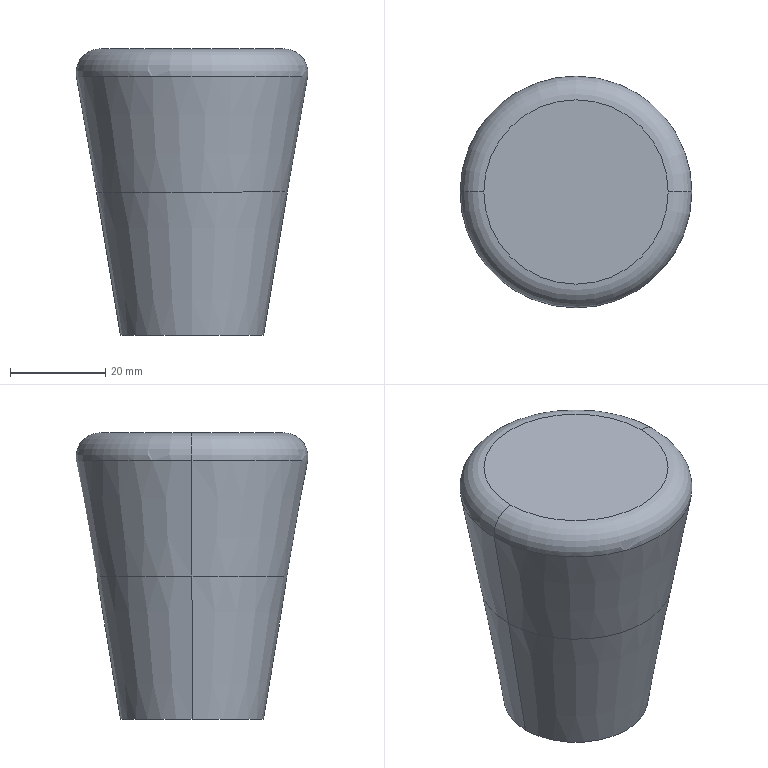Part | SolidWorks | features Extrusion 1, Fillet 1, ICE 1, RevCut 1 | 1 solid | 10 faces | box 48.662 x 48.662 x 60 mm | volume 55216 mm3 | cone 4 | torus 2 | cylinder 2 | plane 2 | commonest cylinder face diameters 30 x2
STEP:
#1=CARTESIAN_POINT('',(-24.255,0.,24.132));
#2=VERTEX_POINT('',#1);
#3=CARTESIAN_POINT('',(24.255,0.,24.132));
#4=VERTEX_POINT('',#3);
#5=CARTESIAN_POINT('',(0.,0.,24.132));
#6=DIRECTION('',(0.,0.,-1.));
#7=DIRECTION('',(1.,0.,0.));
#8=AXIS2_PLACEMENT_3D('',#5,#6,#7);
#9=CIRCLE('',#8,24.255);
#10=EDGE_CURVE('',#2,#4,#9,.T.);
#11=ORIENTED_EDGE('',*,*,#10,.F.);
#12=CARTESIAN_POINT('',(-19.331,0.,30.));
#13=VERTEX_POINT('',#12);
#14=CARTESIAN_POINT('',(-19.331,0.,25.));
#15=DIRECTION('',(0.,1.,0.));
#16=DIRECTION('',(-1.,0.,0.));
#17=AXIS2_PLACEMENT_3D('',#14,#15,#16);
#18=CIRCLE('',#17,5.);
#19=EDGE_CURVE('',#2,#13,#18,.T.);
#20=ORIENTED_EDGE('',*,*,#19,.T.);
#21=CARTESIAN_POINT('',(19.331,0.,30.));
#22=VERTEX_POINT('',#21);
#23=CARTESIAN_POINT('',(0.,0.,30.));
#24=DIRECTION('',(0.,0.,1.));
#25=DIRECTION('',(1.,0.,0.));
#26=AXIS2_PLACEMENT_3D('',#23,#24,#25);
#27=CIRCLE('',#26,19.331);
#28=EDGE_CURVE('',#22,#13,#27,.T.);
#29=ORIENTED_EDGE('',*,*,#28,.F.);
#30=CARTESIAN_POINT('',(19.331,0.,25.));
#31=DIRECTION('',(0.,-1.,0.));
#32=DIRECTION('',(0.,0.,-1.));
#33=AXIS2_PLACEMENT_3D('',#30,#31,#32);
#34=CIRCLE('',#33,5.);
#35=EDGE_CURVE('',#4,#22,#34,.T.);
#36=ORIENTED_EDGE('',*,*,#35,.F.);
#37=EDGE_LOOP('',(#11,#20,#29,#36));
#38=FACE_OUTER_BOUND('',#37,.T.);
#39=CARTESIAN_POINT('',(0.,0.,25.));
#40=DIRECTION('',(0.,0.,1.));
#41=DIRECTION('',(1.,0.,0.));
#42=AXIS2_PLACEMENT_3D('',#39,#40,#41);
#43=TOROIDAL_SURFACE('',#42,19.331,5.);
#44=ADVANCED_FACE('',(#38),#43,.T.);
#45=CARTESIAN_POINT('',(-15.,0.,-30.));
#46=VERTEX_POINT('',#45);
#47=CARTESIAN_POINT('',(15.,0.,-30.));
#48=VERTEX_POINT('',#47);
#49=CARTESIAN_POINT('',(0.,0.,-30.));
#50=DIRECTION('',(0.,0.,1.));
#51=DIRECTION('',(1.,0.,0.));
#52=AXIS2_PLACEMENT_3D('',#49,#50,#51);
#53=CIRCLE('',#52,15.);
#54=EDGE_CURVE('',#46,#48,#53,.T.);
#55=ORIENTED_EDGE('',*,*,#54,.F.);
#56=CARTESIAN_POINT('',(-15.,0.,0.));
#57=VERTEX_POINT('',#56);
#58=CARTESIAN_POINT('',(-15.,0.,-30.));
#59=DIRECTION('',(0.,0.,1.));
#60=VECTOR('',#59,1000.);
#61=LINE('',#58,#60);
#62=EDGE_CURVE('',#46,#57,#61,.T.);
#63=ORIENTED_EDGE('',*,*,#62,.T.);
#64=CARTESIAN_POINT('',(15.,0.,0.));
#65=VERTEX_POINT('',#64);
#66=CARTESIAN_POINT('',(0.,0.,0.));
#67=DIRECTION('',(0.,0.,1.));
#68=DIRECTION('',(1.,0.,0.));
#69=AXIS2_PLACEMENT_3D('',#66,#67,#68);
#70=CIRCLE('',#69,15.);
#71=EDGE_CURVE('',#57,#65,#70,.T.);
#72=ORIENTED_EDGE('',*,*,#71,.T.);
#73=CARTESIAN_POINT('',(15.,0.,-30.));
#74=DIRECTION('',(0.,0.,1.));
#75=VECTOR('',#74,1000.);
#76=LINE('',#73,#75);
#77=EDGE_CURVE('',#48,#65,#76,.T.);
#78=ORIENTED_EDGE('',*,*,#77,.F.);
#79=EDGE_LOOP('',(#55,#63,#72,#78));
#80=FACE_OUTER_BOUND('',#79,.T.);
#81=CARTESIAN_POINT('',(0.,0.,-30.));
#82=DIRECTION('',(0.,0.,1.));
#83=DIRECTION('',(1.,0.,0.));
#84=AXIS2_PLACEMENT_3D('',#81,#82,#83);
#85=CYLINDRICAL_SURFACE('',#84,15.);
#86=ADVANCED_FACE('',(#80),#85,.F.);
#87=CARTESIAN_POINT('',(0.,0.,-30.));
#88=DIRECTION('',(0.,0.,1.));
#89=DIRECTION('',(1.,0.,0.));
#90=AXIS2_PLACEMENT_3D('',#87,#88,#89);
#91=CIRCLE('',#90,15.);
#92=EDGE_CURVE('',#48,#46,#91,.T.);
#93=ORIENTED_EDGE('',*,*,#92,.T.);
#94=CARTESIAN_POINT('',(-20.,0.,0.));
#95=VERTEX_POINT('',#94);
#96=CARTESIAN_POINT('',(-15.,0.,-30.));
#97=DIRECTION('',(-0.1644,0.,0.9864));
#98=VECTOR('',#97,1000.);
#99=LINE('',#96,#98);
#100=EDGE_CURVE('',#46,#95,#99,.T.);
#101=ORIENTED_EDGE('',*,*,#100,.T.);
#102=CARTESIAN_POINT('',(20.,0.,0.));
#103=VERTEX_POINT('',#102);
#104=CARTESIAN_POINT('',(0.,0.,0.));
#105=DIRECTION('',(0.,0.,1.));
#106=DIRECTION('',(1.,0.,0.));
#107=AXIS2_PLACEMENT_3D('',#104,#105,#106);
#108=CIRCLE('',#107,20.);
#109=EDGE_CURVE('',#103,#95,#108,.T.);
#110=ORIENTED_EDGE('',*,*,#109,.F.);
#111=CARTESIAN_POINT('',(15.,0.,-30.));
#112=DIRECTION('',(0.1644,0.,0.9864));
#113=VECTOR('',#112,1000.);
#114=LINE('',#111,#113);
#115=EDGE_CURVE('',#48,#103,#114,.T.);
#116=ORIENTED_EDGE('',*,*,#115,.F.);
#117=EDGE_LOOP('',(#93,#101,#110,#116));
#118=FACE_OUTER_BOUND('',#117,.T.);
#119=CARTESIAN_POINT('',(0.,0.,-30.));
#120=DIRECTION('',(0.,0.,1.));
#121=DIRECTION('',(1.,0.,0.));
#122=AXIS2_PLACEMENT_3D('',#119,#120,#121);
#123=CONICAL_SURFACE('',#122,15.,0.1651);
#124=ADVANCED_FACE('',(#118),#123,.T.);
#125=ORIENTED_EDGE('',*,*,#109,.T.);
#126=CARTESIAN_POINT('',(-20.,0.,0.));
#127=DIRECTION('',(-0.1736,0.,0.9848));
#128=VECTOR('',#127,1000.);
#129=LINE('',#126,#128);
#130=EDGE_CURVE('',#95,#2,#129,.T.);
#131=ORIENTED_EDGE('',*,*,#130,.T.);
#132=ORIENTED_EDGE('',*,*,#10,.T.);
#133=CARTESIAN_POINT('',(20.,0.,0.));
#134=DIRECTION('',(0.1736,0.,0.9848));
#135=VECTOR('',#134,1000.);
#136=LINE('',#133,#135);
#137=EDGE_CURVE('',#103,#4,#136,.T.);
#138=ORIENTED_EDGE('',*,*,#137,.F.);
#139=EDGE_LOOP('',(#125,#131,#132,#138));
#140=FACE_OUTER_BOUND('',#139,.T.);
#141=CARTESIAN_POINT('',(0.,0.,0.));
#142=DIRECTION('',(0.,0.,1.));
#143=DIRECTION('',(1.,0.,0.));
#144=AXIS2_PLACEMENT_3D('',#141,#142,#143);
#145=CONICAL_SURFACE('',#144,20.,0.1745);
#146=ADVANCED_FACE('',(#140),#145,.T.);
#147=ORIENTED_EDGE('',*,*,#130,.F.);
#148=CARTESIAN_POINT('',(0.,0.,0.));
#149=DIRECTION('',(0.,0.,1.));
#150=DIRECTION('',(1.,0.,0.));
#151=AXIS2_PLACEMENT_3D('',#148,#149,#150);
#152=CIRCLE('',#151,20.);
#153=EDGE_CURVE('',#95,#103,#152,.T.);
#154=ORIENTED_EDGE('',*,*,#153,.T.);
#155=ORIENTED_EDGE('',*,*,#137,.T.);
#156=CARTESIAN_POINT('',(0.,0.,24.132));
#157=DIRECTION('',(0.,0.,-1.));
#158=DIRECTION('',(1.,0.,0.));
#159=AXIS2_PLACEMENT_3D('',#156,#157,#158);
#160=CIRCLE('',#159,24.255);
#161=EDGE_CURVE('',#4,#2,#160,.T.);
#162=ORIENTED_EDGE('',*,*,#161,.T.);
#163=EDGE_LOOP('',(#147,#154,#155,#162));
#164=FACE_OUTER_BOUND('',#163,.T.);
#165=CARTESIAN_POINT('',(0.,0.,0.));
#166=DIRECTION('',(0.,0.,1.));
#167=DIRECTION('',(1.,0.,0.));
#168=AXIS2_PLACEMENT_3D('',#165,#166,#167);
#169=CONICAL_SURFACE('',#168,20.,0.1745);
#170=ADVANCED_FACE('',(#164),#169,.T.);
#171=ORIENTED_EDGE('',*,*,#28,.T.);
#172=CARTESIAN_POINT('',(0.,0.,30.));
#173=DIRECTION('',(0.,0.,1.));
#174=DIRECTION('',(1.,0.,0.));
#175=AXIS2_PLACEMENT_3D('',#172,#173,#174);
#176=CIRCLE('',#175,19.331);
#177=EDGE_CURVE('',#13,#22,#176,.T.);
#178=ORIENTED_EDGE('',*,*,#177,.T.);
#179=EDGE_LOOP('',(#171,#178));
#180=FACE_OUTER_BOUND('',#179,.T.);
#181=CARTESIAN_POINT('',(0.,0.,30.));
#182=DIRECTION('',(0.,0.,1.));
#183=DIRECTION('',(1.,0.,0.));
#184=AXIS2_PLACEMENT_3D('',#181,#182,#183);
#185=PLANE('',#184);
#186=ADVANCED_FACE('',(#180),#185,.T.);
#187=ORIENTED_EDGE('',*,*,#100,.F.);
#188=ORIENTED_EDGE('',*,*,#54,.T.);
#189=ORIENTED_EDGE('',*,*,#115,.T.);
#190=ORIENTED_EDGE('',*,*,#153,.F.);
#191=EDGE_LOOP('',(#187,#188,#189,#190));
#192=FACE_OUTER_BOUND('',#191,.T.);
#193=CARTESIAN_POINT('',(0.,0.,-30.));
#194=DIRECTION('',(0.,0.,1.));
#195=DIRECTION('',(1.,0.,0.));
#196=AXIS2_PLACEMENT_3D('',#193,#194,#195);
#197=CONICAL_SURFACE('',#196,15.,0.1651);
#198=ADVANCED_FACE('',(#192),#197,.T.);
#199=CARTESIAN_POINT('',(0.,0.,0.));
#200=DIRECTION('',(0.,0.,1.));
#201=DIRECTION('',(1.,0.,0.));
#202=AXIS2_PLACEMENT_3D('',#199,#200,#201);
#203=CIRCLE('',#202,15.);
#204=EDGE_CURVE('',#65,#57,#203,.T.);
#205=ORIENTED_EDGE('',*,*,#204,.F.);
#206=ORIENTED_EDGE('',*,*,#71,.F.);
#207=EDGE_LOOP('',(#205,#206));
#208=FACE_OUTER_BOUND('',#207,.T.);
#209=CARTESIAN_POINT('',(0.,0.,0.));
#210=DIRECTION('',(0.,0.,1.));
#211=DIRECTION('',(1.,0.,0.));
#212=AXIS2_PLACEMENT_3D('',#209,#210,#211);
#213=PLANE('',#212);
#214=ADVANCED_FACE('',(#208),#213,.F.);
#215=ORIENTED_EDGE('',*,*,#62,.F.);
#216=ORIENTED_EDGE('',*,*,#92,.F.);
#217=ORIENTED_EDGE('',*,*,#77,.T.);
#218=ORIENTED_EDGE('',*,*,#204,.T.);
#219=EDGE_LOOP('',(#215,#216,#217,#218));
#220=FACE_OUTER_BOUND('',#219,.T.);
#221=CARTESIAN_POINT('',(0.,0.,-30.));
#222=DIRECTION('',(0.,0.,1.));
#223=DIRECTION('',(1.,0.,0.));
#224=AXIS2_PLACEMENT_3D('',#221,#222,#223);
#225=CYLINDRICAL_SURFACE('',#224,15.);
#226=ADVANCED_FACE('',(#220),#225,.F.);
#227=ORIENTED_EDGE('',*,*,#19,.F.);
#228=ORIENTED_EDGE('',*,*,#161,.F.);
#229=ORIENTED_EDGE('',*,*,#35,.T.);
#230=ORIENTED_EDGE('',*,*,#177,.F.);
#231=EDGE_LOOP('',(#227,#228,#229,#230));
#232=FACE_OUTER_BOUND('',#231,.T.);
#233=CARTESIAN_POINT('',(0.,0.,25.));
#234=DIRECTION('',(0.,0.,1.));
#235=DIRECTION('',(1.,0.,0.));
#236=AXIS2_PLACEMENT_3D('',#233,#234,#235);
#237=TOROIDAL_SURFACE('',#236,19.331,5.);
#238=ADVANCED_FACE('',(#232),#237,.T.);
#239=CLOSED_SHELL('',(#44,#86,#124,#146,#170,#186,#198,#214,#226,#238));
#240=MANIFOLD_SOLID_BREP('',#239);
#241=CARTESIAN_POINT('',(0.,0.,0.));
#242=DIRECTION('',(0.,0.,1.));
#243=DIRECTION('',(1.,0.,0.));
#244=AXIS2_PLACEMENT_3D('',#241,#242,#243);
#245=(LENGTH_UNIT()NAMED_UNIT(*)SI_UNIT(.MILLI.,.METRE.));
#246=UNCERTAINTY_MEASURE_WITH_UNIT(LENGTH_MEASURE(0.00001),#245,'','');
#247=(NAMED_UNIT(*)PLANE_ANGLE_UNIT()SI_UNIT($,.RADIAN.));
#248=(NAMED_UNIT(*)SI_UNIT($,.STERADIAN.)SOLID_ANGLE_UNIT());
#249=(GEOMETRIC_REPRESENTATION_CONTEXT(3)GLOBAL_UNCERTAINTY_ASSIGNED_CONTEXT((#246))GLOBAL_UNIT_ASSIGNED_CONTEXT((#245,#247,#248))REPRESENTATION_CONTEXT('',''));
#250=ADVANCED_BREP_SHAPE_REPRESENTATION('',(#240,#244),#249);